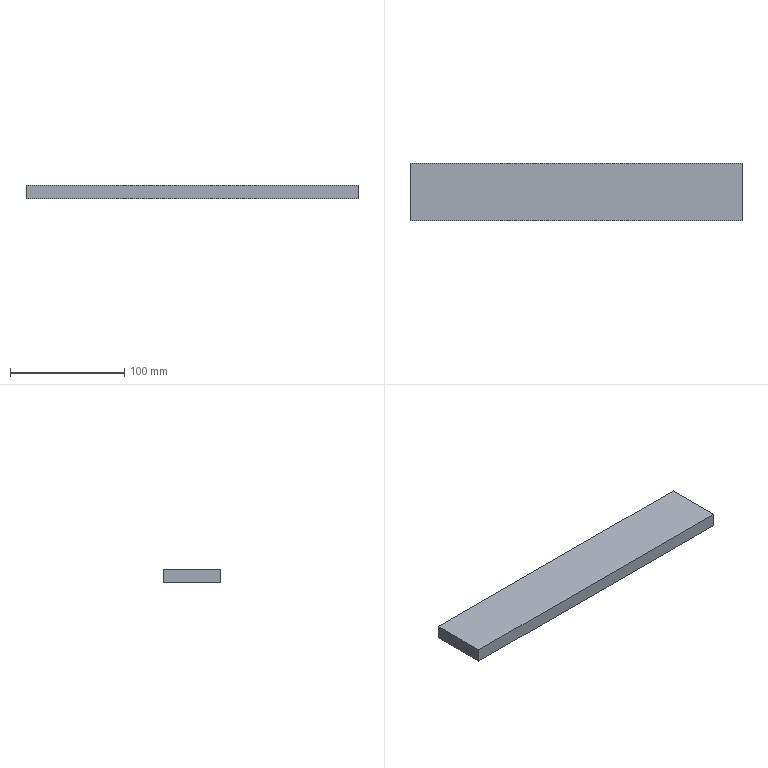Part | SolidWorks | features Extrusion 1 | 1 solid | 6 faces | box 290 x 50 x 12 mm | volume 174000 mm3 | plane 6
STEP:
#1=CARTESIAN_POINT('',(0.,50.,0.));
#2=VERTEX_POINT('',#1);
#3=CARTESIAN_POINT('',(0.,0.,0.));
#4=VERTEX_POINT('',#3);
#5=CARTESIAN_POINT('',(0.,0.,0.));
#6=DIRECTION('',(0.,-1.,0.));
#7=VECTOR('',#6,1000.);
#8=LINE('',#5,#7);
#9=EDGE_CURVE('',#2,#4,#8,.T.);
#10=ORIENTED_EDGE('',*,*,#9,.T.);
#11=CARTESIAN_POINT('',(0.,0.,12.));
#12=VERTEX_POINT('',#11);
#13=CARTESIAN_POINT('',(0.,0.,12.));
#14=DIRECTION('',(0.,0.,-1.));
#15=VECTOR('',#14,1000.);
#16=LINE('',#13,#15);
#17=EDGE_CURVE('',#12,#4,#16,.T.);
#18=ORIENTED_EDGE('',*,*,#17,.F.);
#19=CARTESIAN_POINT('',(0.,50.,12.));
#20=VERTEX_POINT('',#19);
#21=CARTESIAN_POINT('',(0.,0.,12.));
#22=DIRECTION('',(0.,-1.,0.));
#23=VECTOR('',#22,1000.);
#24=LINE('',#21,#23);
#25=EDGE_CURVE('',#20,#12,#24,.T.);
#26=ORIENTED_EDGE('',*,*,#25,.F.);
#27=CARTESIAN_POINT('',(0.,50.,12.));
#28=DIRECTION('',(0.,0.,-1.));
#29=VECTOR('',#28,1000.);
#30=LINE('',#27,#29);
#31=EDGE_CURVE('',#20,#2,#30,.T.);
#32=ORIENTED_EDGE('',*,*,#31,.T.);
#33=EDGE_LOOP('',(#10,#18,#26,#32));
#34=FACE_OUTER_BOUND('',#33,.T.);
#35=CARTESIAN_POINT('',(0.,0.,12.));
#36=DIRECTION('',(1.,0.,0.));
#37=DIRECTION('',(0.,0.,-1.));
#38=AXIS2_PLACEMENT_3D('',#35,#36,#37);
#39=PLANE('',#38);
#40=ADVANCED_FACE('',(#34),#39,.F.);
#41=CARTESIAN_POINT('',(290.,0.,0.));
#42=VERTEX_POINT('',#41);
#43=CARTESIAN_POINT('',(0.,0.,0.));
#44=DIRECTION('',(1.,0.,0.));
#45=VECTOR('',#44,1000.);
#46=LINE('',#43,#45);
#47=EDGE_CURVE('',#4,#42,#46,.T.);
#48=ORIENTED_EDGE('',*,*,#47,.T.);
#49=CARTESIAN_POINT('',(290.,0.,12.));
#50=VERTEX_POINT('',#49);
#51=CARTESIAN_POINT('',(290.,0.,12.));
#52=DIRECTION('',(0.,0.,-1.));
#53=VECTOR('',#52,1000.);
#54=LINE('',#51,#53);
#55=EDGE_CURVE('',#50,#42,#54,.T.);
#56=ORIENTED_EDGE('',*,*,#55,.F.);
#57=CARTESIAN_POINT('',(0.,0.,12.));
#58=DIRECTION('',(1.,0.,0.));
#59=VECTOR('',#58,1000.);
#60=LINE('',#57,#59);
#61=EDGE_CURVE('',#12,#50,#60,.T.);
#62=ORIENTED_EDGE('',*,*,#61,.F.);
#63=ORIENTED_EDGE('',*,*,#17,.T.);
#64=EDGE_LOOP('',(#48,#56,#62,#63));
#65=FACE_OUTER_BOUND('',#64,.T.);
#66=CARTESIAN_POINT('',(0.,0.,12.));
#67=DIRECTION('',(0.,1.,0.));
#68=DIRECTION('',(0.,0.,1.));
#69=AXIS2_PLACEMENT_3D('',#66,#67,#68);
#70=PLANE('',#69);
#71=ADVANCED_FACE('',(#65),#70,.F.);
#72=CARTESIAN_POINT('',(290.,50.,0.));
#73=VERTEX_POINT('',#72);
#74=CARTESIAN_POINT('',(290.,0.,0.));
#75=DIRECTION('',(0.,1.,0.));
#76=VECTOR('',#75,1000.);
#77=LINE('',#74,#76);
#78=EDGE_CURVE('',#42,#73,#77,.T.);
#79=ORIENTED_EDGE('',*,*,#78,.T.);
#80=CARTESIAN_POINT('',(290.,50.,12.));
#81=VERTEX_POINT('',#80);
#82=CARTESIAN_POINT('',(290.,50.,12.));
#83=DIRECTION('',(0.,0.,-1.));
#84=VECTOR('',#83,1000.);
#85=LINE('',#82,#84);
#86=EDGE_CURVE('',#81,#73,#85,.T.);
#87=ORIENTED_EDGE('',*,*,#86,.F.);
#88=CARTESIAN_POINT('',(290.,0.,12.));
#89=DIRECTION('',(0.,1.,0.));
#90=VECTOR('',#89,1000.);
#91=LINE('',#88,#90);
#92=EDGE_CURVE('',#50,#81,#91,.T.);
#93=ORIENTED_EDGE('',*,*,#92,.F.);
#94=ORIENTED_EDGE('',*,*,#55,.T.);
#95=EDGE_LOOP('',(#79,#87,#93,#94));
#96=FACE_OUTER_BOUND('',#95,.T.);
#97=CARTESIAN_POINT('',(290.,0.,12.));
#98=DIRECTION('',(-1.,0.,0.));
#99=DIRECTION('',(0.,0.,1.));
#100=AXIS2_PLACEMENT_3D('',#97,#98,#99);
#101=PLANE('',#100);
#102=ADVANCED_FACE('',(#96),#101,.F.);
#103=CARTESIAN_POINT('',(0.,50.,0.));
#104=DIRECTION('',(-1.,0.,0.));
#105=VECTOR('',#104,1000.);
#106=LINE('',#103,#105);
#107=EDGE_CURVE('',#73,#2,#106,.T.);
#108=ORIENTED_EDGE('',*,*,#107,.T.);
#109=ORIENTED_EDGE('',*,*,#31,.F.);
#110=CARTESIAN_POINT('',(0.,50.,12.));
#111=DIRECTION('',(-1.,0.,0.));
#112=VECTOR('',#111,1000.);
#113=LINE('',#110,#112);
#114=EDGE_CURVE('',#81,#20,#113,.T.);
#115=ORIENTED_EDGE('',*,*,#114,.F.);
#116=ORIENTED_EDGE('',*,*,#86,.T.);
#117=EDGE_LOOP('',(#108,#109,#115,#116));
#118=FACE_OUTER_BOUND('',#117,.T.);
#119=CARTESIAN_POINT('',(0.,50.,12.));
#120=DIRECTION('',(0.,-1.,0.));
#121=DIRECTION('',(0.,0.,-1.));
#122=AXIS2_PLACEMENT_3D('',#119,#120,#121);
#123=PLANE('',#122);
#124=ADVANCED_FACE('',(#118),#123,.F.);
#125=ORIENTED_EDGE('',*,*,#25,.T.);
#126=ORIENTED_EDGE('',*,*,#61,.T.);
#127=ORIENTED_EDGE('',*,*,#92,.T.);
#128=ORIENTED_EDGE('',*,*,#114,.T.);
#129=EDGE_LOOP('',(#125,#126,#127,#128));
#130=FACE_OUTER_BOUND('',#129,.T.);
#131=CARTESIAN_POINT('',(0.,0.,12.));
#132=DIRECTION('',(0.,0.,-1.));
#133=DIRECTION('',(-1.,0.,0.));
#134=AXIS2_PLACEMENT_3D('',#131,#132,#133);
#135=PLANE('',#134);
#136=ADVANCED_FACE('',(#130),#135,.F.);
#137=ORIENTED_EDGE('',*,*,#9,.F.);
#138=ORIENTED_EDGE('',*,*,#107,.F.);
#139=ORIENTED_EDGE('',*,*,#78,.F.);
#140=ORIENTED_EDGE('',*,*,#47,.F.);
#141=EDGE_LOOP('',(#137,#138,#139,#140));
#142=FACE_OUTER_BOUND('',#141,.T.);
#143=CARTESIAN_POINT('',(0.,0.,0.));
#144=DIRECTION('',(0.,0.,-1.));
#145=DIRECTION('',(-1.,0.,0.));
#146=AXIS2_PLACEMENT_3D('',#143,#144,#145);
#147=PLANE('',#146);
#148=ADVANCED_FACE('',(#142),#147,.T.);
#149=CLOSED_SHELL('',(#40,#71,#102,#124,#136,#148));
#150=MANIFOLD_SOLID_BREP('',#149);
#151=CARTESIAN_POINT('',(0.,0.,0.));
#152=DIRECTION('',(0.,0.,1.));
#153=DIRECTION('',(1.,0.,0.));
#154=AXIS2_PLACEMENT_3D('',#151,#152,#153);
#155=(LENGTH_UNIT()NAMED_UNIT(*)SI_UNIT(.MILLI.,.METRE.));
#156=UNCERTAINTY_MEASURE_WITH_UNIT(LENGTH_MEASURE(0.00001),#155,'','');
#157=(NAMED_UNIT(*)PLANE_ANGLE_UNIT()SI_UNIT($,.RADIAN.));
#158=(NAMED_UNIT(*)SI_UNIT($,.STERADIAN.)SOLID_ANGLE_UNIT());
#159=(GEOMETRIC_REPRESENTATION_CONTEXT(3)GLOBAL_UNCERTAINTY_ASSIGNED_CONTEXT((#156))GLOBAL_UNIT_ASSIGNED_CONTEXT((#155,#157,#158))REPRESENTATION_CONTEXT('',''));
#160=ADVANCED_BREP_SHAPE_REPRESENTATION('',(#150,#154),#159);